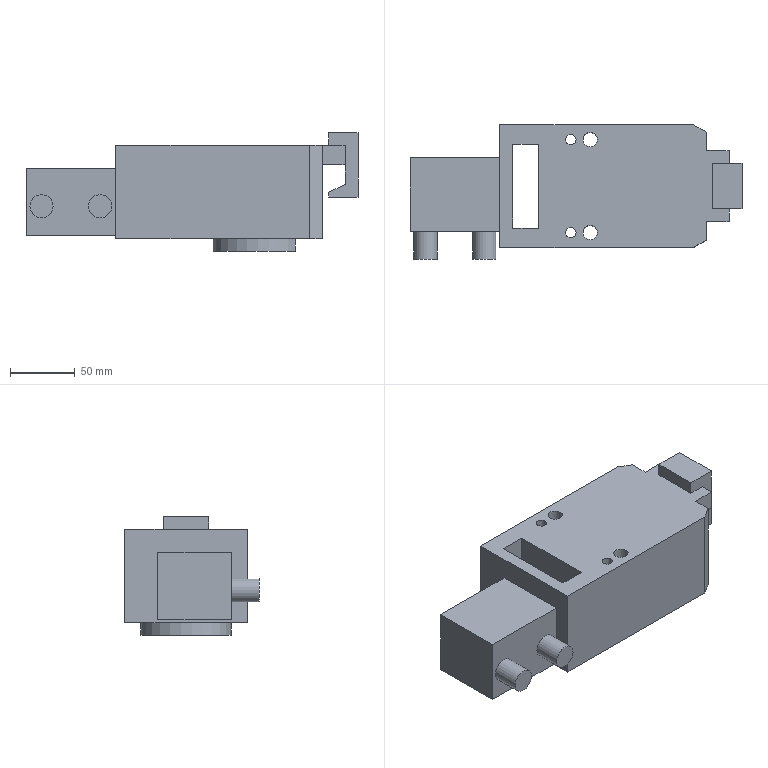Part | NX | features solid 2 | 1 solid | 46 faces | box 257 x 104 x 92 mm | volume 1265438 mm3 | plane 37 | cylinder 9 | commonest cylinder face diameters 8 x2 11 x2 17 x2 18 x2 70 x1
STEP:
#1=CARTESIAN_POINT('',(509.903,-203.405,153.));
#2=VERTEX_POINT('',#1);
#3=CARTESIAN_POINT('',(509.903,-164.213,153.));
#4=VERTEX_POINT('',#3);
#5=CARTESIAN_POINT('',(509.903,-183.809,153.));
#6=DIRECTION('',(0.,1.,0.));
#7=VECTOR('',#6,1000.);
#8=LINE('',#5,#7);
#9=EDGE_CURVE('',#2,#4,#8,.T.);
#10=ORIENTED_EDGE('',*,*,#9,.T.);
#11=CARTESIAN_POINT('',(480.903,-183.809,153.));
#12=DIRECTION('',(0.,0.,1.));
#13=DIRECTION('',(-1.,0.,0.));
#14=AXIS2_PLACEMENT_3D('',#11,#12,#13);
#15=CIRCLE('',#14,35.);
#16=EDGE_CURVE('',#4,#2,#15,.T.);
#17=ORIENTED_EDGE('',*,*,#16,.T.);
#18=EDGE_LOOP('',(#10,#17));
#19=FACE_BOUND('',#18,.T.);
#20=CARTESIAN_POINT('',(400.903,-216.309,153.));
#21=VERTEX_POINT('',#20);
#22=CARTESIAN_POINT('',(380.903,-216.309,153.));
#23=VERTEX_POINT('',#22);
#24=CARTESIAN_POINT('',(400.903,-216.309,153.));
#25=DIRECTION('',(-1.,0.,0.));
#26=VECTOR('',#25,1000.);
#27=LINE('',#24,#26);
#28=EDGE_CURVE('',#21,#23,#27,.T.);
#29=ORIENTED_EDGE('',*,*,#28,.F.);
#30=CARTESIAN_POINT('',(400.903,-151.309,153.));
#31=VERTEX_POINT('',#30);
#32=CARTESIAN_POINT('',(400.903,-156.809,153.));
#33=DIRECTION('',(0.,-1.,0.));
#34=VECTOR('',#33,1000.);
#35=LINE('',#32,#34);
#36=EDGE_CURVE('',#31,#21,#35,.T.);
#37=ORIENTED_EDGE('',*,*,#36,.F.);
#38=CARTESIAN_POINT('',(380.903,-151.309,153.));
#39=VERTEX_POINT('',#38);
#40=CARTESIAN_POINT('',(400.903,-151.309,153.));
#41=DIRECTION('',(-1.,0.,0.));
#42=VECTOR('',#41,1000.);
#43=LINE('',#40,#42);
#44=EDGE_CURVE('',#31,#39,#43,.T.);
#45=ORIENTED_EDGE('',*,*,#44,.T.);
#46=CARTESIAN_POINT('',(380.903,-156.809,153.));
#47=DIRECTION('',(0.,1.,0.));
#48=VECTOR('',#47,1000.);
#49=LINE('',#46,#48);
#50=EDGE_CURVE('',#23,#39,#49,.T.);
#51=ORIENTED_EDGE('',*,*,#50,.F.);
#52=EDGE_LOOP('',(#29,#37,#45,#51));
#53=FACE_BOUND('',#52,.T.);
#54=CARTESIAN_POINT('',(520.903,-231.309,153.));
#55=VERTEX_POINT('',#54);
#56=CARTESIAN_POINT('',(370.903,-231.309,153.));
#57=VERTEX_POINT('',#56);
#58=CARTESIAN_POINT('',(450.903,-231.309,153.));
#59=DIRECTION('',(-1.,0.,0.));
#60=VECTOR('',#59,1000.);
#61=LINE('',#58,#60);
#62=EDGE_CURVE('',#55,#57,#61,.T.);
#63=ORIENTED_EDGE('',*,*,#62,.T.);
#64=CARTESIAN_POINT('',(370.903,-136.309,153.));
#65=VERTEX_POINT('',#64);
#66=CARTESIAN_POINT('',(370.903,-156.809,153.));
#67=DIRECTION('',(0.,-1.,0.));
#68=VECTOR('',#67,1000.);
#69=LINE('',#66,#68);
#70=EDGE_CURVE('',#65,#57,#69,.T.);
#71=ORIENTED_EDGE('',*,*,#70,.F.);
#72=CARTESIAN_POINT('',(520.903,-136.309,153.));
#73=VERTEX_POINT('',#72);
#74=CARTESIAN_POINT('',(450.903,-136.309,153.));
#75=DIRECTION('',(-1.,0.,0.));
#76=VECTOR('',#75,1000.);
#77=LINE('',#74,#76);
#78=EDGE_CURVE('',#73,#65,#77,.T.);
#79=ORIENTED_EDGE('',*,*,#78,.F.);
#80=CARTESIAN_POINT('',(530.903,-142.082,153.));
#81=VERTEX_POINT('',#80);
#82=CARTESIAN_POINT('',(550.903,-153.629,153.));
#83=DIRECTION('',(0.866,-0.5,0.));
#84=VECTOR('',#83,1000.);
#85=LINE('',#82,#84);
#86=EDGE_CURVE('',#81,#73,#85,.F.);
#87=ORIENTED_EDGE('',*,*,#86,.F.);
#88=CARTESIAN_POINT('',(530.903,-225.535,153.));
#89=VERTEX_POINT('',#88);
#90=CARTESIAN_POINT('',(530.903,-178.809,153.));
#91=DIRECTION('',(0.,1.,0.));
#92=VECTOR('',#91,1000.);
#93=LINE('',#90,#92);
#94=EDGE_CURVE('',#89,#81,#93,.T.);
#95=ORIENTED_EDGE('',*,*,#94,.F.);
#96=CARTESIAN_POINT('',(520.903,-231.309,153.));
#97=DIRECTION('',(0.866,0.5,0.));
#98=VECTOR('',#97,1000.);
#99=LINE('',#96,#98);
#100=EDGE_CURVE('',#55,#89,#99,.T.);
#101=ORIENTED_EDGE('',*,*,#100,.F.);
#102=EDGE_LOOP('',(#63,#71,#79,#87,#95,#101));
#103=FACE_BOUND('',#102,.T.);
#104=CARTESIAN_POINT('',(429.903,-219.809,153.));
#105=VERTEX_POINT('',#104);
#106=CARTESIAN_POINT('',(425.903,-219.809,153.));
#107=DIRECTION('',(0.,0.,-1.));
#108=DIRECTION('',(1.,0.,0.));
#109=AXIS2_PLACEMENT_3D('',#106,#107,#108);
#110=CIRCLE('',#109,4.);
#111=EDGE_CURVE('',#105,#105,#110,.F.);
#112=ORIENTED_EDGE('',*,*,#111,.T.);
#113=EDGE_LOOP('',(#112));
#114=FACE_BOUND('',#113,.T.);
#115=CARTESIAN_POINT('',(449.403,-219.809,153.));
#116=VERTEX_POINT('',#115);
#117=CARTESIAN_POINT('',(440.903,-219.809,153.));
#118=DIRECTION('',(0.,0.,-1.));
#119=DIRECTION('',(1.,0.,0.));
#120=AXIS2_PLACEMENT_3D('',#117,#118,#119);
#121=CIRCLE('',#120,8.5);
#122=EDGE_CURVE('',#116,#116,#121,.T.);
#123=ORIENTED_EDGE('',*,*,#122,.F.);
#124=EDGE_LOOP('',(#123));
#125=FACE_BOUND('',#124,.T.);
#126=CARTESIAN_POINT('',(449.403,-147.809,153.));
#127=VERTEX_POINT('',#126);
#128=CARTESIAN_POINT('',(440.903,-147.809,153.));
#129=DIRECTION('',(0.,0.,-1.));
#130=DIRECTION('',(1.,0.,0.));
#131=AXIS2_PLACEMENT_3D('',#128,#129,#130);
#132=CIRCLE('',#131,8.5);
#133=EDGE_CURVE('',#127,#127,#132,.T.);
#134=ORIENTED_EDGE('',*,*,#133,.F.);
#135=EDGE_LOOP('',(#134));
#136=FACE_BOUND('',#135,.T.);
#137=CARTESIAN_POINT('',(429.903,-147.809,153.));
#138=VERTEX_POINT('',#137);
#139=CARTESIAN_POINT('',(425.903,-147.809,153.));
#140=DIRECTION('',(0.,0.,-1.));
#141=DIRECTION('',(1.,0.,0.));
#142=AXIS2_PLACEMENT_3D('',#139,#140,#141);
#143=CIRCLE('',#142,4.);
#144=EDGE_CURVE('',#138,#138,#143,.F.);
#145=ORIENTED_EDGE('',*,*,#144,.T.);
#146=EDGE_LOOP('',(#145));
#147=FACE_BOUND('',#146,.T.);
#148=CARTESIAN_POINT('',(400.903,-156.809,153.));
#149=DIRECTION('',(0.,0.,-1.));
#150=DIRECTION('',(1.,0.,0.));
#151=AXIS2_PLACEMENT_3D('',#148,#149,#150);
#152=PLANE('',#151);
#153=ADVANCED_FACE('',(#19,#53,#103,#114,#125,#136,#147),#152,.T.);
#154=CARTESIAN_POINT('',(400.903,-151.309,225.));
#155=VERTEX_POINT('',#154);
#156=CARTESIAN_POINT('',(400.903,-216.309,225.));
#157=VERTEX_POINT('',#156);
#158=CARTESIAN_POINT('',(400.903,-156.809,225.));
#159=DIRECTION('',(0.,-1.,0.));
#160=VECTOR('',#159,1000.);
#161=LINE('',#158,#160);
#162=EDGE_CURVE('',#155,#157,#161,.T.);
#163=ORIENTED_EDGE('',*,*,#162,.T.);
#164=CARTESIAN_POINT('',(380.903,-216.309,225.));
#165=VERTEX_POINT('',#164);
#166=CARTESIAN_POINT('',(385.903,-216.309,225.));
#167=DIRECTION('',(1.,0.,0.));
#168=VECTOR('',#167,1000.);
#169=LINE('',#166,#168);
#170=EDGE_CURVE('',#157,#165,#169,.F.);
#171=ORIENTED_EDGE('',*,*,#170,.T.);
#172=CARTESIAN_POINT('',(380.903,-151.309,225.));
#173=VERTEX_POINT('',#172);
#174=CARTESIAN_POINT('',(380.903,-156.809,225.));
#175=DIRECTION('',(0.,1.,0.));
#176=VECTOR('',#175,1000.);
#177=LINE('',#174,#176);
#178=EDGE_CURVE('',#165,#173,#177,.T.);
#179=ORIENTED_EDGE('',*,*,#178,.T.);
#180=CARTESIAN_POINT('',(385.903,-151.309,225.));
#181=DIRECTION('',(1.,0.,0.));
#182=VECTOR('',#181,1000.);
#183=LINE('',#180,#182);
#184=EDGE_CURVE('',#155,#173,#183,.F.);
#185=ORIENTED_EDGE('',*,*,#184,.F.);
#186=EDGE_LOOP('',(#163,#171,#179,#185));
#187=FACE_BOUND('',#186,.T.);
#188=CARTESIAN_POINT('',(535.903,-201.309,225.));
#189=VERTEX_POINT('',#188);
#190=CARTESIAN_POINT('',(535.903,-166.309,225.));
#191=VERTEX_POINT('',#190);
#192=CARTESIAN_POINT('',(535.903,-156.809,225.));
#193=DIRECTION('',(0.,-1.,0.));
#194=VECTOR('',#193,1000.);
#195=LINE('',#192,#194);
#196=EDGE_CURVE('',#189,#191,#195,.F.);
#197=ORIENTED_EDGE('',*,*,#196,.T.);
#198=CARTESIAN_POINT('',(548.403,-166.309,225.));
#199=VERTEX_POINT('',#198);
#200=CARTESIAN_POINT('',(568.403,-166.309,225.));
#201=DIRECTION('',(1.,0.,0.));
#202=VECTOR('',#201,1000.);
#203=LINE('',#200,#202);
#204=EDGE_CURVE('',#199,#191,#203,.F.);
#205=ORIENTED_EDGE('',*,*,#204,.F.);
#206=CARTESIAN_POINT('',(548.403,-156.309,225.));
#207=VERTEX_POINT('',#206);
#208=CARTESIAN_POINT('',(548.403,-156.809,225.));
#209=DIRECTION('',(0.,1.,0.));
#210=VECTOR('',#209,1000.);
#211=LINE('',#208,#210);
#212=EDGE_CURVE('',#199,#207,#211,.T.);
#213=ORIENTED_EDGE('',*,*,#212,.T.);
#214=CARTESIAN_POINT('',(530.903,-156.309,225.));
#215=VERTEX_POINT('',#214);
#216=CARTESIAN_POINT('',(578.403,-156.309,225.));
#217=DIRECTION('',(1.,0.,0.));
#218=VECTOR('',#217,1000.);
#219=LINE('',#216,#218);
#220=EDGE_CURVE('',#215,#207,#219,.T.);
#221=ORIENTED_EDGE('',*,*,#220,.F.);
#222=CARTESIAN_POINT('',(530.903,-142.082,225.));
#223=VERTEX_POINT('',#222);
#224=CARTESIAN_POINT('',(530.903,-178.809,225.));
#225=DIRECTION('',(0.,1.,0.));
#226=VECTOR('',#225,1000.);
#227=LINE('',#224,#226);
#228=EDGE_CURVE('',#215,#223,#227,.T.);
#229=ORIENTED_EDGE('',*,*,#228,.T.);
#230=CARTESIAN_POINT('',(520.903,-136.309,225.));
#231=VERTEX_POINT('',#230);
#232=CARTESIAN_POINT('',(550.903,-153.629,225.));
#233=DIRECTION('',(-0.866,0.5,0.));
#234=VECTOR('',#233,1000.);
#235=LINE('',#232,#234);
#236=EDGE_CURVE('',#231,#223,#235,.F.);
#237=ORIENTED_EDGE('',*,*,#236,.F.);
#238=CARTESIAN_POINT('',(370.903,-136.309,225.));
#239=VERTEX_POINT('',#238);
#240=CARTESIAN_POINT('',(400.903,-136.309,225.));
#241=DIRECTION('',(-1.,0.,0.));
#242=VECTOR('',#241,1000.);
#243=LINE('',#240,#242);
#244=EDGE_CURVE('',#231,#239,#243,.T.);
#245=ORIENTED_EDGE('',*,*,#244,.T.);
#246=CARTESIAN_POINT('',(370.903,-231.309,225.));
#247=VERTEX_POINT('',#246);
#248=CARTESIAN_POINT('',(370.903,-156.809,225.));
#249=DIRECTION('',(0.,-1.,0.));
#250=VECTOR('',#249,1000.);
#251=LINE('',#248,#250);
#252=EDGE_CURVE('',#239,#247,#251,.T.);
#253=ORIENTED_EDGE('',*,*,#252,.T.);
#254=CARTESIAN_POINT('',(520.903,-231.309,225.));
#255=VERTEX_POINT('',#254);
#256=CARTESIAN_POINT('',(400.903,-231.309,225.));
#257=DIRECTION('',(-1.,0.,0.));
#258=VECTOR('',#257,1000.);
#259=LINE('',#256,#258);
#260=EDGE_CURVE('',#255,#247,#259,.T.);
#261=ORIENTED_EDGE('',*,*,#260,.F.);
#262=CARTESIAN_POINT('',(530.903,-225.535,225.));
#263=VERTEX_POINT('',#262);
#264=CARTESIAN_POINT('',(520.903,-231.309,225.));
#265=DIRECTION('',(-0.866,-0.5,0.));
#266=VECTOR('',#265,1000.);
#267=LINE('',#264,#266);
#268=EDGE_CURVE('',#263,#255,#267,.T.);
#269=ORIENTED_EDGE('',*,*,#268,.F.);
#270=CARTESIAN_POINT('',(530.903,-211.309,225.));
#271=VERTEX_POINT('',#270);
#272=CARTESIAN_POINT('',(530.903,-178.809,225.));
#273=DIRECTION('',(0.,1.,0.));
#274=VECTOR('',#273,1000.);
#275=LINE('',#272,#274);
#276=EDGE_CURVE('',#263,#271,#275,.T.);
#277=ORIENTED_EDGE('',*,*,#276,.T.);
#278=CARTESIAN_POINT('',(548.403,-211.309,225.));
#279=VERTEX_POINT('',#278);
#280=CARTESIAN_POINT('',(578.403,-211.309,225.));
#281=DIRECTION('',(1.,0.,0.));
#282=VECTOR('',#281,1000.);
#283=LINE('',#280,#282);
#284=EDGE_CURVE('',#271,#279,#283,.T.);
#285=ORIENTED_EDGE('',*,*,#284,.T.);
#286=CARTESIAN_POINT('',(548.403,-201.309,225.));
#287=VERTEX_POINT('',#286);
#288=CARTESIAN_POINT('',(548.403,-156.809,225.));
#289=DIRECTION('',(0.,1.,0.));
#290=VECTOR('',#289,1000.);
#291=LINE('',#288,#290);
#292=EDGE_CURVE('',#279,#287,#291,.T.);
#293=ORIENTED_EDGE('',*,*,#292,.T.);
#294=CARTESIAN_POINT('',(568.403,-201.309,225.));
#295=DIRECTION('',(1.,0.,0.));
#296=VECTOR('',#295,1000.);
#297=LINE('',#294,#296);
#298=EDGE_CURVE('',#287,#189,#297,.F.);
#299=ORIENTED_EDGE('',*,*,#298,.T.);
#300=EDGE_LOOP('',(#197,#205,#213,#221,#229,#237,#245,#253,#261,#269,#277,#285,#293,#299));
#301=FACE_BOUND('',#300,.T.);
#302=CARTESIAN_POINT('',(446.403,-219.809,225.));
#303=VERTEX_POINT('',#302);
#304=CARTESIAN_POINT('',(440.903,-219.809,225.));
#305=DIRECTION('',(0.,0.,-1.));
#306=DIRECTION('',(1.,0.,0.));
#307=AXIS2_PLACEMENT_3D('',#304,#305,#306);
#308=CIRCLE('',#307,5.5);
#309=EDGE_CURVE('',#303,#303,#308,.F.);
#310=ORIENTED_EDGE('',*,*,#309,.F.);
#311=EDGE_LOOP('',(#310));
#312=FACE_BOUND('',#311,.T.);
#313=CARTESIAN_POINT('',(429.903,-219.809,225.));
#314=VERTEX_POINT('',#313);
#315=CARTESIAN_POINT('',(425.903,-219.809,225.));
#316=DIRECTION('',(0.,0.,1.));
#317=DIRECTION('',(1.,0.,0.));
#318=AXIS2_PLACEMENT_3D('',#315,#316,#317);
#319=CIRCLE('',#318,4.);
#320=EDGE_CURVE('',#314,#314,#319,.T.);
#321=ORIENTED_EDGE('',*,*,#320,.F.);
#322=EDGE_LOOP('',(#321));
#323=FACE_BOUND('',#322,.T.);
#324=CARTESIAN_POINT('',(429.903,-147.809,225.));
#325=VERTEX_POINT('',#324);
#326=CARTESIAN_POINT('',(425.903,-147.809,225.));
#327=DIRECTION('',(0.,0.,1.));
#328=DIRECTION('',(1.,0.,0.));
#329=AXIS2_PLACEMENT_3D('',#326,#327,#328);
#330=CIRCLE('',#329,4.);
#331=EDGE_CURVE('',#325,#325,#330,.T.);
#332=ORIENTED_EDGE('',*,*,#331,.F.);
#333=EDGE_LOOP('',(#332));
#334=FACE_BOUND('',#333,.T.);
#335=CARTESIAN_POINT('',(446.403,-147.809,225.));
#336=VERTEX_POINT('',#335);
#337=CARTESIAN_POINT('',(440.903,-147.809,225.));
#338=DIRECTION('',(0.,0.,-1.));
#339=DIRECTION('',(1.,0.,0.));
#340=AXIS2_PLACEMENT_3D('',#337,#338,#339);
#341=CIRCLE('',#340,5.5);
#342=EDGE_CURVE('',#336,#336,#341,.F.);
#343=ORIENTED_EDGE('',*,*,#342,.F.);
#344=EDGE_LOOP('',(#343));
#345=FACE_BOUND('',#344,.T.);
#346=CARTESIAN_POINT('',(400.903,-156.809,225.));
#347=DIRECTION('',(0.,0.,-1.));
#348=DIRECTION('',(1.,0.,0.));
#349=AXIS2_PLACEMENT_3D('',#346,#347,#348);
#350=PLANE('',#349);
#351=ADVANCED_FACE('',(#187,#301,#312,#323,#334,#345),#350,.F.);
#352=ORIENTED_EDGE('',*,*,#94,.T.);
#353=CARTESIAN_POINT('',(530.903,-142.082,225.));
#354=DIRECTION('',(0.,0.,1.));
#355=VECTOR('',#354,1000.);
#356=LINE('',#353,#355);
#357=EDGE_CURVE('',#223,#81,#356,.F.);
#358=ORIENTED_EDGE('',*,*,#357,.F.);
#359=ORIENTED_EDGE('',*,*,#228,.F.);
#360=CARTESIAN_POINT('',(530.903,-156.309,210.));
#361=VERTEX_POINT('',#360);
#362=CARTESIAN_POINT('',(530.903,-156.309,225.));
#363=DIRECTION('',(0.,0.,1.));
#364=VECTOR('',#363,1000.);
#365=LINE('',#362,#364);
#366=EDGE_CURVE('',#215,#361,#365,.F.);
#367=ORIENTED_EDGE('',*,*,#366,.T.);
#368=CARTESIAN_POINT('',(530.903,-211.309,210.));
#369=VERTEX_POINT('',#368);
#370=CARTESIAN_POINT('',(530.903,-231.309,210.));
#371=DIRECTION('',(0.,-1.,0.));
#372=VECTOR('',#371,1000.);
#373=LINE('',#370,#372);
#374=EDGE_CURVE('',#361,#369,#373,.T.);
#375=ORIENTED_EDGE('',*,*,#374,.T.);
#376=CARTESIAN_POINT('',(530.903,-211.309,225.));
#377=DIRECTION('',(0.,0.,1.));
#378=VECTOR('',#377,1000.);
#379=LINE('',#376,#378);
#380=EDGE_CURVE('',#369,#271,#379,.T.);
#381=ORIENTED_EDGE('',*,*,#380,.T.);
#382=ORIENTED_EDGE('',*,*,#276,.F.);
#383=CARTESIAN_POINT('',(530.903,-225.535,225.));
#384=DIRECTION('',(0.,0.,1.));
#385=VECTOR('',#384,1000.);
#386=LINE('',#383,#385);
#387=EDGE_CURVE('',#89,#263,#386,.T.);
#388=ORIENTED_EDGE('',*,*,#387,.F.);
#389=EDGE_LOOP('',(#352,#358,#359,#367,#375,#381,#382,#388));
#390=FACE_BOUND('',#389,.T.);
#391=CARTESIAN_POINT('',(530.903,-178.809,225.));
#392=DIRECTION('',(1.,0.,0.));
#393=DIRECTION('',(0.,1.,0.));
#394=AXIS2_PLACEMENT_3D('',#391,#392,#393);
#395=PLANE('',#394);
#396=ADVANCED_FACE('',(#390),#395,.T.);
#397=CARTESIAN_POINT('',(400.903,-216.309,225.));
#398=DIRECTION('',(0.,0.,-1.));
#399=VECTOR('',#398,1000.);
#400=LINE('',#397,#399);
#401=EDGE_CURVE('',#157,#21,#400,.T.);
#402=ORIENTED_EDGE('',*,*,#401,.F.);
#403=ORIENTED_EDGE('',*,*,#162,.F.);
#404=CARTESIAN_POINT('',(400.903,-151.309,225.));
#405=DIRECTION('',(0.,0.,-1.));
#406=VECTOR('',#405,1000.);
#407=LINE('',#404,#406);
#408=EDGE_CURVE('',#155,#31,#407,.T.);
#409=ORIENTED_EDGE('',*,*,#408,.T.);
#410=ORIENTED_EDGE('',*,*,#36,.T.);
#411=EDGE_LOOP('',(#402,#403,#409,#410));
#412=FACE_BOUND('',#411,.T.);
#413=CARTESIAN_POINT('',(400.903,-156.809,225.));
#414=DIRECTION('',(-1.,0.,0.));
#415=DIRECTION('',(0.,-1.,0.));
#416=AXIS2_PLACEMENT_3D('',#413,#414,#415);
#417=PLANE('',#416);
#418=ADVANCED_FACE('',(#412),#417,.T.);
#419=CARTESIAN_POINT('',(370.903,-218.809,207.5));
#420=VERTEX_POINT('',#419);
#421=CARTESIAN_POINT('',(370.903,-161.809,207.5));
#422=VERTEX_POINT('',#421);
#423=CARTESIAN_POINT('',(370.903,-241.309,207.5));
#424=DIRECTION('',(0.,1.,0.));
#425=VECTOR('',#424,1000.);
#426=LINE('',#423,#425);
#427=EDGE_CURVE('',#420,#422,#426,.T.);
#428=ORIENTED_EDGE('',*,*,#427,.F.);
#429=CARTESIAN_POINT('',(370.903,-218.809,155.5));
#430=VERTEX_POINT('',#429);
#431=CARTESIAN_POINT('',(370.903,-218.809,196.));
#432=DIRECTION('',(0.,0.,-1.));
#433=VECTOR('',#432,1000.);
#434=LINE('',#431,#433);
#435=EDGE_CURVE('',#420,#430,#434,.T.);
#436=ORIENTED_EDGE('',*,*,#435,.T.);
#437=CARTESIAN_POINT('',(370.903,-161.809,155.5));
#438=VERTEX_POINT('',#437);
#439=CARTESIAN_POINT('',(370.903,-146.809,155.5));
#440=DIRECTION('',(0.,-1.,0.));
#441=VECTOR('',#440,1000.);
#442=LINE('',#439,#441);
#443=EDGE_CURVE('',#438,#430,#442,.T.);
#444=ORIENTED_EDGE('',*,*,#443,.F.);
#445=CARTESIAN_POINT('',(370.903,-161.809,196.));
#446=DIRECTION('',(0.,0.,-1.));
#447=VECTOR('',#446,1000.);
#448=LINE('',#445,#447);
#449=EDGE_CURVE('',#422,#438,#448,.T.);
#450=ORIENTED_EDGE('',*,*,#449,.F.);
#451=EDGE_LOOP('',(#428,#436,#444,#450));
#452=FACE_BOUND('',#451,.T.);
#453=CARTESIAN_POINT('',(370.903,-231.309,225.));
#454=DIRECTION('',(0.,0.,-1.));
#455=VECTOR('',#454,1000.);
#456=LINE('',#453,#455);
#457=EDGE_CURVE('',#247,#57,#456,.T.);
#458=ORIENTED_EDGE('',*,*,#457,.F.);
#459=ORIENTED_EDGE('',*,*,#252,.F.);
#460=CARTESIAN_POINT('',(370.903,-136.309,225.));
#461=DIRECTION('',(0.,0.,-1.));
#462=VECTOR('',#461,1000.);
#463=LINE('',#460,#462);
#464=EDGE_CURVE('',#239,#65,#463,.T.);
#465=ORIENTED_EDGE('',*,*,#464,.T.);
#466=ORIENTED_EDGE('',*,*,#70,.T.);
#467=EDGE_LOOP('',(#458,#459,#465,#466));
#468=FACE_BOUND('',#467,.T.);
#469=CARTESIAN_POINT('',(370.903,-121.309,193.));
#470=DIRECTION('',(1.,0.,0.));
#471=DIRECTION('',(0.,0.,-1.));
#472=AXIS2_PLACEMENT_3D('',#469,#470,#471);
#473=PLANE('',#472);
#474=ADVANCED_FACE('',(#452,#468),#473,.F.);
#475=ORIENTED_EDGE('',*,*,#50,.T.);
#476=CARTESIAN_POINT('',(380.903,-151.309,193.));
#477=DIRECTION('',(0.,0.,1.));
#478=VECTOR('',#477,1000.);
#479=LINE('',#476,#478);
#480=EDGE_CURVE('',#39,#173,#479,.T.);
#481=ORIENTED_EDGE('',*,*,#480,.T.);
#482=ORIENTED_EDGE('',*,*,#178,.F.);
#483=CARTESIAN_POINT('',(380.903,-216.309,193.));
#484=DIRECTION('',(0.,0.,-1.));
#485=VECTOR('',#484,1000.);
#486=LINE('',#483,#485);
#487=EDGE_CURVE('',#165,#23,#486,.T.);
#488=ORIENTED_EDGE('',*,*,#487,.T.);
#489=EDGE_LOOP('',(#475,#481,#482,#488));
#490=FACE_BOUND('',#489,.T.);
#491=CARTESIAN_POINT('',(380.903,-235.809,193.));
#492=DIRECTION('',(-1.,0.,0.));
#493=DIRECTION('',(0.,0.,1.));
#494=AXIS2_PLACEMENT_3D('',#491,#492,#493);
#495=PLANE('',#494);
#496=ADVANCED_FACE('',(#490),#495,.F.);
#497=CARTESIAN_POINT('',(558.403,-201.309,185.));
#498=VERTEX_POINT('',#497);
#499=CARTESIAN_POINT('',(558.403,-166.309,185.));
#500=VERTEX_POINT('',#499);
#501=CARTESIAN_POINT('',(558.403,-231.309,185.));
#502=DIRECTION('',(0.,1.,0.));
#503=VECTOR('',#502,1000.);
#504=LINE('',#501,#503);
#505=EDGE_CURVE('',#498,#500,#504,.T.);
#506=ORIENTED_EDGE('',*,*,#505,.T.);
#507=CARTESIAN_POINT('',(558.403,-166.309,235.));
#508=VERTEX_POINT('',#507);
#509=CARTESIAN_POINT('',(558.403,-166.309,225.));
#510=DIRECTION('',(0.,0.,-1.));
#511=VECTOR('',#510,1000.);
#512=LINE('',#509,#511);
#513=EDGE_CURVE('',#508,#500,#512,.T.);
#514=ORIENTED_EDGE('',*,*,#513,.F.);
#515=CARTESIAN_POINT('',(558.403,-201.309,235.));
#516=VERTEX_POINT('',#515);
#517=CARTESIAN_POINT('',(558.403,-231.309,235.));
#518=DIRECTION('',(0.,1.,0.));
#519=VECTOR('',#518,1000.);
#520=LINE('',#517,#519);
#521=EDGE_CURVE('',#516,#508,#520,.T.);
#522=ORIENTED_EDGE('',*,*,#521,.F.);
#523=CARTESIAN_POINT('',(558.403,-201.309,225.));
#524=DIRECTION('',(0.,0.,1.));
#525=VECTOR('',#524,1000.);
#526=LINE('',#523,#525);
#527=EDGE_CURVE('',#516,#498,#526,.F.);
#528=ORIENTED_EDGE('',*,*,#527,.T.);
#529=EDGE_LOOP('',(#506,#514,#522,#528));
#530=FACE_BOUND('',#529,.T.);
#531=CARTESIAN_POINT('',(558.403,-231.309,225.));
#532=DIRECTION('',(1.,0.,0.));
#533=DIRECTION('',(0.,1.,0.));
#534=AXIS2_PLACEMENT_3D('',#531,#532,#533);
#535=PLANE('',#534);
#536=ADVANCED_FACE('',(#530),#535,.T.);
#537=ORIENTED_EDGE('',*,*,#521,.T.);
#538=CARTESIAN_POINT('',(535.903,-166.309,235.));
#539=VERTEX_POINT('',#538);
#540=CARTESIAN_POINT('',(578.403,-166.309,235.));
#541=DIRECTION('',(-1.,0.,0.));
#542=VECTOR('',#541,1000.);
#543=LINE('',#540,#542);
#544=EDGE_CURVE('',#508,#539,#543,.T.);
#545=ORIENTED_EDGE('',*,*,#544,.T.);
#546=CARTESIAN_POINT('',(535.903,-201.309,235.));
#547=VERTEX_POINT('',#546);
#548=CARTESIAN_POINT('',(535.903,-231.309,235.));
#549=DIRECTION('',(0.,-1.,0.));
#550=VECTOR('',#549,1000.);
#551=LINE('',#548,#550);
#552=EDGE_CURVE('',#547,#539,#551,.F.);
#553=ORIENTED_EDGE('',*,*,#552,.F.);
#554=CARTESIAN_POINT('',(578.403,-201.309,235.));
#555=DIRECTION('',(1.,0.,0.));
#556=VECTOR('',#555,1000.);
#557=LINE('',#554,#556);
#558=EDGE_CURVE('',#516,#547,#557,.F.);
#559=ORIENTED_EDGE('',*,*,#558,.F.);
#560=EDGE_LOOP('',(#537,#545,#553,#559));
#561=FACE_BOUND('',#560,.T.);
#562=CARTESIAN_POINT('',(578.403,-231.309,235.));
#563=DIRECTION('',(0.,0.,-1.));
#564=DIRECTION('',(-1.,0.,0.));
#565=AXIS2_PLACEMENT_3D('',#562,#563,#564);
#566=PLANE('',#565);
#567=ADVANCED_FACE('',(#561),#566,.F.);
#568=CARTESIAN_POINT('',(548.403,-211.309,210.));
#569=VERTEX_POINT('',#568);
#570=CARTESIAN_POINT('',(548.403,-201.309,210.));
#571=VERTEX_POINT('',#570);
#572=CARTESIAN_POINT('',(548.403,-231.309,210.));
#573=DIRECTION('',(0.,1.,0.));
#574=VECTOR('',#573,1000.);
#575=LINE('',#572,#574);
#576=EDGE_CURVE('',#569,#571,#575,.T.);
#577=ORIENTED_EDGE('',*,*,#576,.F.);
#578=CARTESIAN_POINT('',(578.403,-211.309,210.));
#579=DIRECTION('',(1.,0.,0.));
#580=VECTOR('',#579,1000.);
#581=LINE('',#578,#580);
#582=EDGE_CURVE('',#369,#569,#581,.T.);
#583=ORIENTED_EDGE('',*,*,#582,.F.);
#584=ORIENTED_EDGE('',*,*,#374,.F.);
#585=CARTESIAN_POINT('',(548.403,-156.309,210.));
#586=VERTEX_POINT('',#585);
#587=CARTESIAN_POINT('',(578.403,-156.309,210.));
#588=DIRECTION('',(-1.,0.,0.));
#589=VECTOR('',#588,1000.);
#590=LINE('',#587,#589);
#591=EDGE_CURVE('',#361,#586,#590,.F.);
#592=ORIENTED_EDGE('',*,*,#591,.T.);
#593=CARTESIAN_POINT('',(548.403,-166.309,210.));
#594=VERTEX_POINT('',#593);
#595=CARTESIAN_POINT('',(548.403,-231.309,210.));
#596=DIRECTION('',(0.,1.,0.));
#597=VECTOR('',#596,1000.);
#598=LINE('',#595,#597);
#599=EDGE_CURVE('',#594,#586,#598,.T.);
#600=ORIENTED_EDGE('',*,*,#599,.F.);
#601=CARTESIAN_POINT('',(548.403,-231.309,210.));
#602=DIRECTION('',(0.,-1.,0.));
#603=VECTOR('',#602,1000.);
#604=LINE('',#601,#603);
#605=EDGE_CURVE('',#571,#594,#604,.F.);
#606=ORIENTED_EDGE('',*,*,#605,.F.);
#607=EDGE_LOOP('',(#577,#583,#584,#592,#600,#606));
#608=FACE_BOUND('',#607,.T.);
#609=CARTESIAN_POINT('',(578.403,-231.309,210.));
#610=DIRECTION('',(0.,0.,-1.));
#611=DIRECTION('',(0.,1.,0.));
#612=AXIS2_PLACEMENT_3D('',#609,#610,#611);
#613=PLANE('',#612);
#614=ADVANCED_FACE('',(#608),#613,.T.);
#615=ORIENTED_EDGE('',*,*,#605,.T.);
#616=CARTESIAN_POINT('',(548.403,-166.309,195.));
#617=VERTEX_POINT('',#616);
#618=CARTESIAN_POINT('',(548.403,-166.309,225.));
#619=DIRECTION('',(0.,0.,1.));
#620=VECTOR('',#619,1000.);
#621=LINE('',#618,#620);
#622=EDGE_CURVE('',#594,#617,#621,.F.);
#623=ORIENTED_EDGE('',*,*,#622,.T.);
#624=CARTESIAN_POINT('',(548.403,-201.309,195.));
#625=VERTEX_POINT('',#624);
#626=CARTESIAN_POINT('',(548.403,-138.809,195.));
#627=DIRECTION('',(0.,1.,0.));
#628=VECTOR('',#627,1000.);
#629=LINE('',#626,#628);
#630=EDGE_CURVE('',#617,#625,#629,.F.);
#631=ORIENTED_EDGE('',*,*,#630,.T.);
#632=CARTESIAN_POINT('',(548.403,-201.309,225.));
#633=DIRECTION('',(0.,0.,-1.));
#634=VECTOR('',#633,1000.);
#635=LINE('',#632,#634);
#636=EDGE_CURVE('',#571,#625,#635,.T.);
#637=ORIENTED_EDGE('',*,*,#636,.F.);
#638=EDGE_LOOP('',(#615,#623,#631,#637));
#639=FACE_BOUND('',#638,.T.);
#640=CARTESIAN_POINT('',(548.403,-231.309,225.));
#641=DIRECTION('',(1.,0.,0.));
#642=DIRECTION('',(0.,1.,0.));
#643=AXIS2_PLACEMENT_3D('',#640,#641,#642);
#644=PLANE('',#643);
#645=ADVANCED_FACE('',(#639),#644,.F.);
#646=CARTESIAN_POINT('',(535.903,-201.309,185.));
#647=VERTEX_POINT('',#646);
#648=CARTESIAN_POINT('',(578.403,-201.309,185.));
#649=DIRECTION('',(1.,0.,0.));
#650=VECTOR('',#649,1000.);
#651=LINE('',#648,#650);
#652=EDGE_CURVE('',#498,#647,#651,.F.);
#653=ORIENTED_EDGE('',*,*,#652,.T.);
#654=CARTESIAN_POINT('',(535.903,-166.309,185.));
#655=VERTEX_POINT('',#654);
#656=CARTESIAN_POINT('',(535.903,-231.309,185.));
#657=DIRECTION('',(0.,-1.,0.));
#658=VECTOR('',#657,1000.);
#659=LINE('',#656,#658);
#660=EDGE_CURVE('',#655,#647,#659,.T.);
#661=ORIENTED_EDGE('',*,*,#660,.F.);
#662=CARTESIAN_POINT('',(578.403,-166.309,185.));
#663=DIRECTION('',(-1.,0.,0.));
#664=VECTOR('',#663,1000.);
#665=LINE('',#662,#664);
#666=EDGE_CURVE('',#500,#655,#665,.T.);
#667=ORIENTED_EDGE('',*,*,#666,.F.);
#668=ORIENTED_EDGE('',*,*,#505,.F.);
#669=EDGE_LOOP('',(#653,#661,#667,#668));
#670=FACE_BOUND('',#669,.T.);
#671=CARTESIAN_POINT('',(578.403,-231.309,185.));
#672=DIRECTION('',(0.,0.,-1.));
#673=DIRECTION('',(-1.,0.,0.));
#674=AXIS2_PLACEMENT_3D('',#671,#672,#673);
#675=PLANE('',#674);
#676=ADVANCED_FACE('',(#670),#675,.T.);
#677=CARTESIAN_POINT('',(535.903,-201.309,188.75));
#678=VERTEX_POINT('',#677);
#679=CARTESIAN_POINT('',(568.403,-201.309,205.));
#680=DIRECTION('',(-0.8944,0.,-0.4472));
#681=VECTOR('',#680,1000.);
#682=LINE('',#679,#681);
#683=EDGE_CURVE('',#678,#625,#682,.F.);
#684=ORIENTED_EDGE('',*,*,#683,.T.);
#685=ORIENTED_EDGE('',*,*,#630,.F.);
#686=CARTESIAN_POINT('',(535.903,-166.309,188.75));
#687=VERTEX_POINT('',#686);
#688=CARTESIAN_POINT('',(568.403,-166.309,205.));
#689=DIRECTION('',(-0.8944,0.,-0.4472));
#690=VECTOR('',#689,1000.);
#691=LINE('',#688,#690);
#692=EDGE_CURVE('',#617,#687,#691,.T.);
#693=ORIENTED_EDGE('',*,*,#692,.T.);
#694=CARTESIAN_POINT('',(535.903,-138.809,188.75));
#695=DIRECTION('',(0.,1.,0.));
#696=VECTOR('',#695,1000.);
#697=LINE('',#694,#696);
#698=EDGE_CURVE('',#678,#687,#697,.T.);
#699=ORIENTED_EDGE('',*,*,#698,.F.);
#700=EDGE_LOOP('',(#684,#685,#693,#699));
#701=FACE_BOUND('',#700,.T.);
#702=CARTESIAN_POINT('',(568.403,-138.809,205.));
#703=DIRECTION('',(-0.4472,0.,0.8944));
#704=DIRECTION('',(0.8944,0.,0.4472));
#705=AXIS2_PLACEMENT_3D('',#702,#703,#704);
#706=PLANE('',#705);
#707=ADVANCED_FACE('',(#701),#706,.T.);
#708=ORIENTED_EDGE('',*,*,#698,.T.);
#709=CARTESIAN_POINT('',(535.903,-166.309,225.));
#710=DIRECTION('',(0.,0.,-1.));
#711=VECTOR('',#710,1000.);
#712=LINE('',#709,#711);
#713=EDGE_CURVE('',#687,#655,#712,.T.);
#714=ORIENTED_EDGE('',*,*,#713,.T.);
#715=ORIENTED_EDGE('',*,*,#660,.T.);
#716=CARTESIAN_POINT('',(535.903,-201.309,225.));
#717=DIRECTION('',(0.,0.,-1.));
#718=VECTOR('',#717,1000.);
#719=LINE('',#716,#718);
#720=EDGE_CURVE('',#647,#678,#719,.F.);
#721=ORIENTED_EDGE('',*,*,#720,.T.);
#722=EDGE_LOOP('',(#708,#714,#715,#721));
#723=FACE_BOUND('',#722,.T.);
#724=CARTESIAN_POINT('',(535.903,-231.309,225.));
#725=DIRECTION('',(1.,0.,0.));
#726=DIRECTION('',(0.,1.,0.));
#727=AXIS2_PLACEMENT_3D('',#724,#725,#726);
#728=PLANE('',#727);
#729=ADVANCED_FACE('',(#723),#728,.F.);
#730=ORIENTED_EDGE('',*,*,#552,.T.);
#731=CARTESIAN_POINT('',(535.903,-166.309,225.));
#732=DIRECTION('',(0.,0.,1.));
#733=VECTOR('',#732,1000.);
#734=LINE('',#731,#733);
#735=EDGE_CURVE('',#539,#191,#734,.F.);
#736=ORIENTED_EDGE('',*,*,#735,.T.);
#737=ORIENTED_EDGE('',*,*,#196,.F.);
#738=CARTESIAN_POINT('',(535.903,-201.309,225.));
#739=DIRECTION('',(0.,0.,-1.));
#740=VECTOR('',#739,1000.);
#741=LINE('',#738,#740);
#742=EDGE_CURVE('',#547,#189,#741,.T.);
#743=ORIENTED_EDGE('',*,*,#742,.F.);
#744=EDGE_LOOP('',(#730,#736,#737,#743));
#745=FACE_BOUND('',#744,.T.);
#746=CARTESIAN_POINT('',(535.903,-231.309,225.));
#747=DIRECTION('',(1.,0.,0.));
#748=DIRECTION('',(0.,1.,0.));
#749=AXIS2_PLACEMENT_3D('',#746,#747,#748);
#750=PLANE('',#749);
#751=ADVANCED_FACE('',(#745),#750,.F.);
#752=ORIENTED_EDGE('',*,*,#236,.T.);
#753=ORIENTED_EDGE('',*,*,#357,.T.);
#754=ORIENTED_EDGE('',*,*,#86,.T.);
#755=CARTESIAN_POINT('',(520.903,-136.309,225.));
#756=DIRECTION('',(0.,0.,1.));
#757=VECTOR('',#756,1000.);
#758=LINE('',#755,#757);
#759=EDGE_CURVE('',#73,#231,#758,.T.);
#760=ORIENTED_EDGE('',*,*,#759,.T.);
#761=EDGE_LOOP('',(#752,#753,#754,#760));
#762=FACE_BOUND('',#761,.T.);
#763=CARTESIAN_POINT('',(550.903,-153.629,225.));
#764=DIRECTION('',(-0.5,-0.866,0.));
#765=DIRECTION('',(0.866,-0.5,0.));
#766=AXIS2_PLACEMENT_3D('',#763,#764,#765);
#767=PLANE('',#766);
#768=ADVANCED_FACE('',(#762),#767,.F.);
#769=ORIENTED_EDGE('',*,*,#78,.T.);
#770=ORIENTED_EDGE('',*,*,#464,.F.);
#771=ORIENTED_EDGE('',*,*,#244,.F.);
#772=ORIENTED_EDGE('',*,*,#759,.F.);
#773=EDGE_LOOP('',(#769,#770,#771,#772));
#774=FACE_BOUND('',#773,.T.);
#775=CARTESIAN_POINT('',(450.903,-136.309,225.));
#776=DIRECTION('',(0.,1.,0.));
#777=DIRECTION('',(-1.,0.,0.));
#778=AXIS2_PLACEMENT_3D('',#775,#776,#777);
#779=PLANE('',#778);
#780=ADVANCED_FACE('',(#774),#779,.T.);
#781=ORIENTED_EDGE('',*,*,#144,.F.);
#782=EDGE_LOOP('',(#781));
#783=FACE_BOUND('',#782,.T.);
#784=ORIENTED_EDGE('',*,*,#331,.T.);
#785=EDGE_LOOP('',(#784));
#786=FACE_BOUND('',#785,.T.);
#787=CARTESIAN_POINT('',(425.903,-147.809,225.));
#788=DIRECTION('',(0.,0.,-1.));
#789=DIRECTION('',(1.,0.,0.));
#790=AXIS2_PLACEMENT_3D('',#787,#788,#789);
#791=CYLINDRICAL_SURFACE('',#790,4.);
#792=ADVANCED_FACE('',(#783,#786),#791,.F.);
#793=ORIENTED_EDGE('',*,*,#133,.T.);
#794=EDGE_LOOP('',(#793));
#795=FACE_BOUND('',#794,.T.);
#796=CARTESIAN_POINT('',(449.403,-147.809,166.));
#797=VERTEX_POINT('',#796);
#798=CARTESIAN_POINT('',(440.903,-147.809,166.));
#799=DIRECTION('',(0.,0.,-1.));
#800=DIRECTION('',(1.,0.,0.));
#801=AXIS2_PLACEMENT_3D('',#798,#799,#800);
#802=CIRCLE('',#801,8.5);
#803=EDGE_CURVE('',#797,#797,#802,.T.);
#804=ORIENTED_EDGE('',*,*,#803,.F.);
#805=EDGE_LOOP('',(#804));
#806=FACE_BOUND('',#805,.T.);
#807=CARTESIAN_POINT('',(440.903,-147.809,146.));
#808=DIRECTION('',(0.,0.,-1.));
#809=DIRECTION('',(1.,0.,0.));
#810=AXIS2_PLACEMENT_3D('',#807,#808,#809);
#811=CYLINDRICAL_SURFACE('',#810,8.5);
#812=ADVANCED_FACE('',(#795,#806),#811,.F.);
#813=ORIENTED_EDGE('',*,*,#342,.T.);
#814=EDGE_LOOP('',(#813));
#815=FACE_BOUND('',#814,.T.);
#816=CARTESIAN_POINT('',(446.403,-147.809,166.));
#817=VERTEX_POINT('',#816);
#818=CARTESIAN_POINT('',(440.903,-147.809,166.));
#819=DIRECTION('',(0.,0.,-1.));
#820=DIRECTION('',(1.,0.,0.));
#821=AXIS2_PLACEMENT_3D('',#818,#819,#820);
#822=CIRCLE('',#821,5.5);
#823=EDGE_CURVE('',#817,#817,#822,.F.);
#824=ORIENTED_EDGE('',*,*,#823,.F.);
#825=EDGE_LOOP('',(#824));
#826=FACE_BOUND('',#825,.T.);
#827=CARTESIAN_POINT('',(440.903,-147.809,175.));
#828=DIRECTION('',(0.,0.,-1.));
#829=DIRECTION('',(1.,0.,0.));
#830=AXIS2_PLACEMENT_3D('',#827,#828,#829);
#831=CYLINDRICAL_SURFACE('',#830,5.5);
#832=ADVANCED_FACE('',(#815,#826),#831,.F.);
#833=ORIENTED_EDGE('',*,*,#803,.T.);
#834=EDGE_LOOP('',(#833));
#835=FACE_BOUND('',#834,.T.);
#836=ORIENTED_EDGE('',*,*,#823,.T.);
#837=EDGE_LOOP('',(#836));
#838=FACE_BOUND('',#837,.T.);
#839=CARTESIAN_POINT('',(440.903,-147.809,166.));
#840=DIRECTION('',(0.,0.,-1.));
#841=DIRECTION('',(1.,0.,0.));
#842=AXIS2_PLACEMENT_3D('',#839,#840,#841);
#843=PLANE('',#842);
#844=ADVANCED_FACE('',(#835,#838),#843,.T.);
#845=ORIENTED_EDGE('',*,*,#44,.F.);
#846=ORIENTED_EDGE('',*,*,#408,.F.);
#847=ORIENTED_EDGE('',*,*,#184,.T.);
#848=ORIENTED_EDGE('',*,*,#480,.F.);
#849=EDGE_LOOP('',(#845,#846,#847,#848));
#850=FACE_BOUND('',#849,.T.);
#851=CARTESIAN_POINT('',(385.903,-151.309,193.));
#852=DIRECTION('',(0.,-1.,0.));
#853=DIRECTION('',(0.,0.,-1.));
#854=AXIS2_PLACEMENT_3D('',#851,#852,#853);
#855=PLANE('',#854);
#856=ADVANCED_FACE('',(#850),#855,.T.);
#857=CARTESIAN_POINT('',(548.403,-156.309,225.));
#858=DIRECTION('',(0.,0.,1.));
#859=VECTOR('',#858,1000.);
#860=LINE('',#857,#859);
#861=EDGE_CURVE('',#207,#586,#860,.F.);
#862=ORIENTED_EDGE('',*,*,#861,.F.);
#863=ORIENTED_EDGE('',*,*,#212,.F.);
#864=CARTESIAN_POINT('',(548.403,-166.309,225.));
#865=DIRECTION('',(0.,0.,-1.));
#866=VECTOR('',#865,1000.);
#867=LINE('',#864,#866);
#868=EDGE_CURVE('',#199,#594,#867,.T.);
#869=ORIENTED_EDGE('',*,*,#868,.T.);
#870=ORIENTED_EDGE('',*,*,#599,.T.);
#871=EDGE_LOOP('',(#862,#863,#869,#870));
#872=FACE_BOUND('',#871,.T.);
#873=CARTESIAN_POINT('',(548.403,-261.309,225.));
#874=DIRECTION('',(-1.,0.,0.));
#875=DIRECTION('',(0.,0.,1.));
#876=AXIS2_PLACEMENT_3D('',#873,#874,#875);
#877=PLANE('',#876);
#878=ADVANCED_FACE('',(#872),#877,.F.);
#879=ORIENTED_EDGE('',*,*,#220,.T.);
#880=ORIENTED_EDGE('',*,*,#861,.T.);
#881=ORIENTED_EDGE('',*,*,#591,.F.);
#882=ORIENTED_EDGE('',*,*,#366,.F.);
#883=EDGE_LOOP('',(#879,#880,#881,#882));
#884=FACE_BOUND('',#883,.T.);
#885=CARTESIAN_POINT('',(578.403,-156.309,225.));
#886=DIRECTION('',(0.,-1.,0.));
#887=DIRECTION('',(0.,0.,-1.));
#888=AXIS2_PLACEMENT_3D('',#885,#886,#887);
#889=PLANE('',#888);
#890=ADVANCED_FACE('',(#884),#889,.F.);
#891=ORIENTED_EDGE('',*,*,#713,.F.);
#892=ORIENTED_EDGE('',*,*,#692,.F.);
#893=ORIENTED_EDGE('',*,*,#622,.F.);
#894=ORIENTED_EDGE('',*,*,#868,.F.);
#895=ORIENTED_EDGE('',*,*,#204,.T.);
#896=ORIENTED_EDGE('',*,*,#735,.F.);
#897=ORIENTED_EDGE('',*,*,#544,.F.);
#898=ORIENTED_EDGE('',*,*,#513,.T.);
#899=ORIENTED_EDGE('',*,*,#666,.T.);
#900=EDGE_LOOP('',(#891,#892,#893,#894,#895,#896,#897,#898,#899));
#901=FACE_BOUND('',#900,.T.);
#902=CARTESIAN_POINT('',(578.403,-166.309,225.));
#903=DIRECTION('',(0.,1.,0.));
#904=DIRECTION('',(-1.,0.,0.));
#905=AXIS2_PLACEMENT_3D('',#902,#903,#904);
#906=PLANE('',#905);
#907=ADVANCED_FACE('',(#901),#906,.T.);
#908=ORIENTED_EDGE('',*,*,#720,.F.);
#909=ORIENTED_EDGE('',*,*,#652,.F.);
#910=ORIENTED_EDGE('',*,*,#527,.F.);
#911=ORIENTED_EDGE('',*,*,#558,.T.);
#912=ORIENTED_EDGE('',*,*,#742,.T.);
#913=ORIENTED_EDGE('',*,*,#298,.F.);
#914=CARTESIAN_POINT('',(548.403,-201.309,225.));
#915=DIRECTION('',(0.,0.,1.));
#916=VECTOR('',#915,1000.);
#917=LINE('',#914,#916);
#918=EDGE_CURVE('',#287,#571,#917,.F.);
#919=ORIENTED_EDGE('',*,*,#918,.T.);
#920=ORIENTED_EDGE('',*,*,#636,.T.);
#921=ORIENTED_EDGE('',*,*,#683,.F.);
#922=EDGE_LOOP('',(#908,#909,#910,#911,#912,#913,#919,#920,#921));
#923=FACE_BOUND('',#922,.T.);
#924=CARTESIAN_POINT('',(578.403,-201.309,225.));
#925=DIRECTION('',(0.,1.,0.));
#926=DIRECTION('',(-1.,0.,0.));
#927=AXIS2_PLACEMENT_3D('',#924,#925,#926);
#928=PLANE('',#927);
#929=ADVANCED_FACE('',(#923),#928,.F.);
#930=ORIENTED_EDGE('',*,*,#292,.F.);
#931=CARTESIAN_POINT('',(548.403,-211.309,225.));
#932=DIRECTION('',(0.,0.,-1.));
#933=VECTOR('',#932,1000.);
#934=LINE('',#931,#933);
#935=EDGE_CURVE('',#279,#569,#934,.T.);
#936=ORIENTED_EDGE('',*,*,#935,.T.);
#937=ORIENTED_EDGE('',*,*,#576,.T.);
#938=ORIENTED_EDGE('',*,*,#918,.F.);
#939=EDGE_LOOP('',(#930,#936,#937,#938));
#940=FACE_BOUND('',#939,.T.);
#941=CARTESIAN_POINT('',(548.403,-211.309,225.));
#942=DIRECTION('',(-1.,0.,0.));
#943=DIRECTION('',(0.,0.,1.));
#944=AXIS2_PLACEMENT_3D('',#941,#942,#943);
#945=PLANE('',#944);
#946=ADVANCED_FACE('',(#940),#945,.F.);
#947=ORIENTED_EDGE('',*,*,#935,.F.);
#948=ORIENTED_EDGE('',*,*,#284,.F.);
#949=ORIENTED_EDGE('',*,*,#380,.F.);
#950=ORIENTED_EDGE('',*,*,#582,.T.);
#951=EDGE_LOOP('',(#947,#948,#949,#950));
#952=FACE_BOUND('',#951,.T.);
#953=CARTESIAN_POINT('',(578.403,-211.309,225.));
#954=DIRECTION('',(0.,-1.,0.));
#955=DIRECTION('',(0.,0.,-1.));
#956=AXIS2_PLACEMENT_3D('',#953,#954,#955);
#957=PLANE('',#956);
#958=ADVANCED_FACE('',(#952),#957,.T.);
#959=ORIENTED_EDGE('',*,*,#170,.F.);
#960=ORIENTED_EDGE('',*,*,#401,.T.);
#961=ORIENTED_EDGE('',*,*,#28,.T.);
#962=ORIENTED_EDGE('',*,*,#487,.F.);
#963=EDGE_LOOP('',(#959,#960,#961,#962));
#964=FACE_BOUND('',#963,.T.);
#965=CARTESIAN_POINT('',(385.903,-216.309,193.));
#966=DIRECTION('',(0.,-1.,0.));
#967=DIRECTION('',(0.,0.,-1.));
#968=AXIS2_PLACEMENT_3D('',#965,#966,#967);
#969=PLANE('',#968);
#970=ADVANCED_FACE('',(#964),#969,.F.);
#971=ORIENTED_EDGE('',*,*,#260,.T.);
#972=ORIENTED_EDGE('',*,*,#457,.T.);
#973=ORIENTED_EDGE('',*,*,#62,.F.);
#974=CARTESIAN_POINT('',(520.903,-231.309,135.));
#975=DIRECTION('',(0.,0.,-1.));
#976=VECTOR('',#975,1000.);
#977=LINE('',#974,#976);
#978=EDGE_CURVE('',#255,#55,#977,.T.);
#979=ORIENTED_EDGE('',*,*,#978,.F.);
#980=EDGE_LOOP('',(#971,#972,#973,#979));
#981=FACE_BOUND('',#980,.T.);
#982=CARTESIAN_POINT('',(450.903,-231.309,225.));
#983=DIRECTION('',(0.,1.,0.));
#984=DIRECTION('',(-1.,0.,0.));
#985=AXIS2_PLACEMENT_3D('',#982,#983,#984);
#986=PLANE('',#985);
#987=ADVANCED_FACE('',(#981),#986,.F.);
#988=ORIENTED_EDGE('',*,*,#268,.T.);
#989=ORIENTED_EDGE('',*,*,#978,.T.);
#990=ORIENTED_EDGE('',*,*,#100,.T.);
#991=ORIENTED_EDGE('',*,*,#387,.T.);
#992=EDGE_LOOP('',(#988,#989,#990,#991));
#993=FACE_BOUND('',#992,.T.);
#994=CARTESIAN_POINT('',(520.903,-231.309,225.));
#995=DIRECTION('',(0.5,-0.866,0.));
#996=DIRECTION('',(0.866,0.5,0.));
#997=AXIS2_PLACEMENT_3D('',#994,#995,#996);
#998=PLANE('',#997);
#999=ADVANCED_FACE('',(#993),#998,.T.);
#1000=ORIENTED_EDGE('',*,*,#309,.T.);
#1001=EDGE_LOOP('',(#1000));
#1002=FACE_BOUND('',#1001,.T.);
#1003=CARTESIAN_POINT('',(446.403,-219.809,166.));
#1004=VERTEX_POINT('',#1003);
#1005=CARTESIAN_POINT('',(440.903,-219.809,166.));
#1006=DIRECTION('',(0.,0.,-1.));
#1007=DIRECTION('',(1.,0.,0.));
#1008=AXIS2_PLACEMENT_3D('',#1005,#1006,#1007);
#1009=CIRCLE('',#1008,5.5);
#1010=EDGE_CURVE('',#1004,#1004,#1009,.F.);
#1011=ORIENTED_EDGE('',*,*,#1010,.F.);
#1012=EDGE_LOOP('',(#1011));
#1013=FACE_BOUND('',#1012,.T.);
#1014=CARTESIAN_POINT('',(440.903,-219.809,175.));
#1015=DIRECTION('',(0.,0.,-1.));
#1016=DIRECTION('',(1.,0.,0.));
#1017=AXIS2_PLACEMENT_3D('',#1014,#1015,#1016);
#1018=CYLINDRICAL_SURFACE('',#1017,5.5);
#1019=ADVANCED_FACE('',(#1002,#1013),#1018,.F.);
#1020=ORIENTED_EDGE('',*,*,#111,.F.);
#1021=EDGE_LOOP('',(#1020));
#1022=FACE_BOUND('',#1021,.T.);
#1023=ORIENTED_EDGE('',*,*,#320,.T.);
#1024=EDGE_LOOP('',(#1023));
#1025=FACE_BOUND('',#1024,.T.);
#1026=CARTESIAN_POINT('',(425.903,-219.809,225.));
#1027=DIRECTION('',(0.,0.,-1.));
#1028=DIRECTION('',(1.,0.,0.));
#1029=AXIS2_PLACEMENT_3D('',#1026,#1027,#1028);
#1030=CYLINDRICAL_SURFACE('',#1029,4.);
#1031=ADVANCED_FACE('',(#1022,#1025),#1030,.F.);
#1032=ORIENTED_EDGE('',*,*,#122,.T.);
#1033=EDGE_LOOP('',(#1032));
#1034=FACE_BOUND('',#1033,.T.);
#1035=CARTESIAN_POINT('',(449.403,-219.809,166.));
#1036=VERTEX_POINT('',#1035);
#1037=CARTESIAN_POINT('',(440.903,-219.809,166.));
#1038=DIRECTION('',(0.,0.,-1.));
#1039=DIRECTION('',(1.,0.,0.));
#1040=AXIS2_PLACEMENT_3D('',#1037,#1038,#1039);
#1041=CIRCLE('',#1040,8.5);
#1042=EDGE_CURVE('',#1036,#1036,#1041,.T.);
#1043=ORIENTED_EDGE('',*,*,#1042,.F.);
#1044=EDGE_LOOP('',(#1043));
#1045=FACE_BOUND('',#1044,.T.);
#1046=CARTESIAN_POINT('',(440.903,-219.809,146.));
#1047=DIRECTION('',(0.,0.,-1.));
#1048=DIRECTION('',(1.,0.,0.));
#1049=AXIS2_PLACEMENT_3D('',#1046,#1047,#1048);
#1050=CYLINDRICAL_SURFACE('',#1049,8.5);
#1051=ADVANCED_FACE('',(#1034,#1045),#1050,.F.);
#1052=ORIENTED_EDGE('',*,*,#1042,.T.);
#1053=EDGE_LOOP('',(#1052));
#1054=FACE_BOUND('',#1053,.T.);
#1055=ORIENTED_EDGE('',*,*,#1010,.T.);
#1056=EDGE_LOOP('',(#1055));
#1057=FACE_BOUND('',#1056,.T.);
#1058=CARTESIAN_POINT('',(440.903,-219.809,166.));
#1059=DIRECTION('',(0.,0.,-1.));
#1060=DIRECTION('',(1.,0.,0.));
#1061=AXIS2_PLACEMENT_3D('',#1058,#1059,#1060);
#1062=PLANE('',#1061);
#1063=ADVANCED_FACE('',(#1054,#1057),#1062,.T.);
#1064=CARTESIAN_POINT('',(509.903,-203.405,143.));
#1065=VERTEX_POINT('',#1064);
#1066=CARTESIAN_POINT('',(509.903,-203.405,143.));
#1067=DIRECTION('',(0.,0.,1.));
#1068=VECTOR('',#1067,1000.);
#1069=LINE('',#1066,#1068);
#1070=EDGE_CURVE('',#1065,#2,#1069,.T.);
#1071=ORIENTED_EDGE('',*,*,#1070,.F.);
#1072=CARTESIAN_POINT('',(509.903,-164.213,143.));
#1073=VERTEX_POINT('',#1072);
#1074=CARTESIAN_POINT('',(509.903,-183.809,143.));
#1075=DIRECTION('',(0.,1.,0.));
#1076=VECTOR('',#1075,1000.);
#1077=LINE('',#1074,#1076);
#1078=EDGE_CURVE('',#1065,#1073,#1077,.T.);
#1079=ORIENTED_EDGE('',*,*,#1078,.T.);
#1080=CARTESIAN_POINT('',(509.903,-164.213,143.));
#1081=DIRECTION('',(0.,0.,1.));
#1082=VECTOR('',#1081,1000.);
#1083=LINE('',#1080,#1082);
#1084=EDGE_CURVE('',#4,#1073,#1083,.F.);
#1085=ORIENTED_EDGE('',*,*,#1084,.F.);
#1086=ORIENTED_EDGE('',*,*,#9,.F.);
#1087=EDGE_LOOP('',(#1071,#1079,#1085,#1086));
#1088=FACE_BOUND('',#1087,.T.);
#1089=CARTESIAN_POINT('',(509.903,-183.809,143.));
#1090=DIRECTION('',(1.,0.,0.));
#1091=DIRECTION('',(0.,1.,0.));
#1092=AXIS2_PLACEMENT_3D('',#1089,#1090,#1091);
#1093=PLANE('',#1092);
#1094=ADVANCED_FACE('',(#1088),#1093,.T.);
#1095=ORIENTED_EDGE('',*,*,#16,.F.);
#1096=ORIENTED_EDGE('',*,*,#1084,.T.);
#1097=CARTESIAN_POINT('',(480.903,-183.809,143.));
#1098=DIRECTION('',(0.,0.,1.));
#1099=DIRECTION('',(-1.,0.,0.));
#1100=AXIS2_PLACEMENT_3D('',#1097,#1098,#1099);
#1101=CIRCLE('',#1100,35.);
#1102=EDGE_CURVE('',#1073,#1065,#1101,.T.);
#1103=ORIENTED_EDGE('',*,*,#1102,.T.);
#1104=ORIENTED_EDGE('',*,*,#1070,.T.);
#1105=EDGE_LOOP('',(#1095,#1096,#1103,#1104));
#1106=FACE_BOUND('',#1105,.T.);
#1107=CARTESIAN_POINT('',(480.903,-183.809,143.));
#1108=DIRECTION('',(0.,0.,1.));
#1109=DIRECTION('',(-1.,0.,0.));
#1110=AXIS2_PLACEMENT_3D('',#1107,#1108,#1109);
#1111=CYLINDRICAL_SURFACE('',#1110,35.);
#1112=ADVANCED_FACE('',(#1106),#1111,.T.);
#1113=ORIENTED_EDGE('',*,*,#1078,.F.);
#1114=ORIENTED_EDGE('',*,*,#1102,.F.);
#1115=EDGE_LOOP('',(#1113,#1114));
#1116=FACE_BOUND('',#1115,.T.);
#1117=CARTESIAN_POINT('',(480.903,-183.809,143.));
#1118=DIRECTION('',(0.,0.,1.));
#1119=DIRECTION('',(-1.,0.,0.));
#1120=AXIS2_PLACEMENT_3D('',#1117,#1118,#1119);
#1121=PLANE('',#1120);
#1122=ADVANCED_FACE('',(#1116),#1121,.F.);
#1123=CARTESIAN_POINT('',(322.403,-218.809,178.));
#1124=VERTEX_POINT('',#1123);
#1125=CARTESIAN_POINT('',(313.403,-218.809,178.));
#1126=DIRECTION('',(0.,-1.,0.));
#1127=DIRECTION('',(1.,0.,0.));
#1128=AXIS2_PLACEMENT_3D('',#1125,#1126,#1127);
#1129=CIRCLE('',#1128,9.);
#1130=EDGE_CURVE('',#1124,#1124,#1129,.F.);
#1131=ORIENTED_EDGE('',*,*,#1130,.T.);
#1132=EDGE_LOOP('',(#1131));
#1133=FACE_BOUND('',#1132,.T.);
#1134=CARTESIAN_POINT('',(367.903,-218.809,178.));
#1135=VERTEX_POINT('',#1134);
#1136=CARTESIAN_POINT('',(358.903,-218.809,178.));
#1137=DIRECTION('',(0.,-1.,0.));
#1138=DIRECTION('',(1.,0.,0.));
#1139=AXIS2_PLACEMENT_3D('',#1136,#1137,#1138);
#1140=CIRCLE('',#1139,9.);
#1141=EDGE_CURVE('',#1135,#1135,#1140,.F.);
#1142=ORIENTED_EDGE('',*,*,#1141,.T.);
#1143=EDGE_LOOP('',(#1142));
#1144=FACE_BOUND('',#1143,.T.);
#1145=CARTESIAN_POINT('',(301.403,-218.809,207.5));
#1146=VERTEX_POINT('',#1145);
#1147=CARTESIAN_POINT('',(326.403,-218.809,207.5));
#1148=DIRECTION('',(-1.,0.,0.));
#1149=VECTOR('',#1148,1000.);
#1150=LINE('',#1147,#1149);
#1151=EDGE_CURVE('',#420,#1146,#1150,.T.);
#1152=ORIENTED_EDGE('',*,*,#1151,.T.);
#1153=CARTESIAN_POINT('',(301.403,-218.809,155.5));
#1154=VERTEX_POINT('',#1153);
#1155=CARTESIAN_POINT('',(301.403,-218.809,207.));
#1156=DIRECTION('',(0.,0.,1.));
#1157=VECTOR('',#1156,1000.);
#1158=LINE('',#1155,#1157);
#1159=EDGE_CURVE('',#1146,#1154,#1158,.F.);
#1160=ORIENTED_EDGE('',*,*,#1159,.T.);
#1161=CARTESIAN_POINT('',(326.403,-218.809,155.5));
#1162=DIRECTION('',(1.,0.,0.));
#1163=VECTOR('',#1162,1000.);
#1164=LINE('',#1161,#1163);
#1165=EDGE_CURVE('',#1154,#430,#1164,.T.);
#1166=ORIENTED_EDGE('',*,*,#1165,.T.);
#1167=ORIENTED_EDGE('',*,*,#435,.F.);
#1168=EDGE_LOOP('',(#1152,#1160,#1166,#1167));
#1169=FACE_BOUND('',#1168,.T.);
#1170=CARTESIAN_POINT('',(326.403,-218.809,207.));
#1171=DIRECTION('',(0.,-1.,0.));
#1172=DIRECTION('',(0.,0.,-1.));
#1173=AXIS2_PLACEMENT_3D('',#1170,#1171,#1172);
#1174=PLANE('',#1173);
#1175=ADVANCED_FACE('',(#1133,#1144,#1169),#1174,.T.);
#1176=CARTESIAN_POINT('',(367.903,-240.309,178.));
#1177=VERTEX_POINT('',#1176);
#1178=CARTESIAN_POINT('',(358.903,-240.309,178.));
#1179=DIRECTION('',(0.,-1.,0.));
#1180=DIRECTION('',(1.,0.,0.));
#1181=AXIS2_PLACEMENT_3D('',#1178,#1179,#1180);
#1182=CIRCLE('',#1181,9.);
#1183=EDGE_CURVE('',#1177,#1177,#1182,.F.);
#1184=ORIENTED_EDGE('',*,*,#1183,.F.);
#1185=EDGE_LOOP('',(#1184));
#1186=FACE_BOUND('',#1185,.T.);
#1187=CARTESIAN_POINT('',(358.903,-240.309,178.));
#1188=DIRECTION('',(0.,-1.,0.));
#1189=DIRECTION('',(0.,0.,1.));
#1190=AXIS2_PLACEMENT_3D('',#1187,#1188,#1189);
#1191=PLANE('',#1190);
#1192=ADVANCED_FACE('',(#1186),#1191,.T.);
#1193=ORIENTED_EDGE('',*,*,#1141,.F.);
#1194=EDGE_LOOP('',(#1193));
#1195=FACE_BOUND('',#1194,.T.);
#1196=ORIENTED_EDGE('',*,*,#1183,.T.);
#1197=EDGE_LOOP('',(#1196));
#1198=FACE_BOUND('',#1197,.T.);
#1199=CARTESIAN_POINT('',(358.903,-238.309,178.));
#1200=DIRECTION('',(0.,1.,0.));
#1201=DIRECTION('',(0.,0.,-1.));
#1202=AXIS2_PLACEMENT_3D('',#1199,#1200,#1201);
#1203=CYLINDRICAL_SURFACE('',#1202,9.);
#1204=ADVANCED_FACE('',(#1195,#1198),#1203,.T.);
#1205=CARTESIAN_POINT('',(301.403,-161.809,155.5));
#1206=VERTEX_POINT('',#1205);
#1207=CARTESIAN_POINT('',(301.403,-205.809,155.5));
#1208=DIRECTION('',(0.,-1.,0.));
#1209=VECTOR('',#1208,1000.);
#1210=LINE('',#1207,#1209);
#1211=EDGE_CURVE('',#1154,#1206,#1210,.F.);
#1212=ORIENTED_EDGE('',*,*,#1211,.T.);
#1213=CARTESIAN_POINT('',(405.903,-161.809,155.5));
#1214=DIRECTION('',(-1.,0.,0.));
#1215=VECTOR('',#1214,1000.);
#1216=LINE('',#1213,#1215);
#1217=EDGE_CURVE('',#438,#1206,#1216,.T.);
#1218=ORIENTED_EDGE('',*,*,#1217,.F.);
#1219=ORIENTED_EDGE('',*,*,#443,.T.);
#1220=ORIENTED_EDGE('',*,*,#1165,.F.);
#1221=EDGE_LOOP('',(#1212,#1218,#1219,#1220));
#1222=FACE_BOUND('',#1221,.T.);
#1223=CARTESIAN_POINT('',(405.903,-146.809,155.5));
#1224=DIRECTION('',(0.,0.,-1.));
#1225=DIRECTION('',(1.,0.,0.));
#1226=AXIS2_PLACEMENT_3D('',#1223,#1224,#1225);
#1227=PLANE('',#1226);
#1228=ADVANCED_FACE('',(#1222),#1227,.T.);
#1229=CARTESIAN_POINT('',(301.403,-161.809,207.5));
#1230=VERTEX_POINT('',#1229);
#1231=CARTESIAN_POINT('',(326.403,-161.809,207.5));
#1232=DIRECTION('',(1.,0.,0.));
#1233=VECTOR('',#1232,1000.);
#1234=LINE('',#1231,#1233);
#1235=EDGE_CURVE('',#1230,#422,#1234,.T.);
#1236=ORIENTED_EDGE('',*,*,#1235,.T.);
#1237=ORIENTED_EDGE('',*,*,#449,.T.);
#1238=ORIENTED_EDGE('',*,*,#1217,.T.);
#1239=CARTESIAN_POINT('',(301.403,-161.809,207.));
#1240=DIRECTION('',(0.,0.,1.));
#1241=VECTOR('',#1240,1000.);
#1242=LINE('',#1239,#1241);
#1243=EDGE_CURVE('',#1230,#1206,#1242,.F.);
#1244=ORIENTED_EDGE('',*,*,#1243,.F.);
#1245=EDGE_LOOP('',(#1236,#1237,#1238,#1244));
#1246=FACE_BOUND('',#1245,.T.);
#1247=CARTESIAN_POINT('',(326.403,-161.809,207.));
#1248=DIRECTION('',(0.,-1.,0.));
#1249=DIRECTION('',(0.,0.,-1.));
#1250=AXIS2_PLACEMENT_3D('',#1247,#1248,#1249);
#1251=PLANE('',#1250);
#1252=ADVANCED_FACE('',(#1246),#1251,.F.);
#1253=CARTESIAN_POINT('',(301.403,-205.809,207.5));
#1254=DIRECTION('',(0.,-1.,0.));
#1255=VECTOR('',#1254,1000.);
#1256=LINE('',#1253,#1255);
#1257=EDGE_CURVE('',#1146,#1230,#1256,.F.);
#1258=ORIENTED_EDGE('',*,*,#1257,.F.);
#1259=ORIENTED_EDGE('',*,*,#1151,.F.);
#1260=ORIENTED_EDGE('',*,*,#427,.T.);
#1261=ORIENTED_EDGE('',*,*,#1235,.F.);
#1262=EDGE_LOOP('',(#1258,#1259,#1260,#1261));
#1263=FACE_BOUND('',#1262,.T.);
#1264=CARTESIAN_POINT('',(326.403,-205.809,207.5));
#1265=DIRECTION('',(0.,0.,-1.));
#1266=DIRECTION('',(1.,0.,0.));
#1267=AXIS2_PLACEMENT_3D('',#1264,#1265,#1266);
#1268=PLANE('',#1267);
#1269=ADVANCED_FACE('',(#1263),#1268,.F.);
#1270=CARTESIAN_POINT('',(322.403,-240.309,178.));
#1271=VERTEX_POINT('',#1270);
#1272=CARTESIAN_POINT('',(313.403,-240.309,178.));
#1273=DIRECTION('',(0.,-1.,0.));
#1274=DIRECTION('',(1.,0.,0.));
#1275=AXIS2_PLACEMENT_3D('',#1272,#1273,#1274);
#1276=CIRCLE('',#1275,9.);
#1277=EDGE_CURVE('',#1271,#1271,#1276,.F.);
#1278=ORIENTED_EDGE('',*,*,#1277,.F.);
#1279=EDGE_LOOP('',(#1278));
#1280=FACE_BOUND('',#1279,.T.);
#1281=CARTESIAN_POINT('',(364.903,-240.309,178.));
#1282=DIRECTION('',(0.,-1.,0.));
#1283=DIRECTION('',(0.,0.,1.));
#1284=AXIS2_PLACEMENT_3D('',#1281,#1282,#1283);
#1285=PLANE('',#1284);
#1286=ADVANCED_FACE('',(#1280),#1285,.T.);
#1287=ORIENTED_EDGE('',*,*,#1130,.F.);
#1288=EDGE_LOOP('',(#1287));
#1289=FACE_BOUND('',#1288,.T.);
#1290=ORIENTED_EDGE('',*,*,#1277,.T.);
#1291=EDGE_LOOP('',(#1290));
#1292=FACE_BOUND('',#1291,.T.);
#1293=CARTESIAN_POINT('',(313.403,-238.309,178.));
#1294=DIRECTION('',(0.,1.,0.));
#1295=DIRECTION('',(0.,0.,-1.));
#1296=AXIS2_PLACEMENT_3D('',#1293,#1294,#1295);
#1297=CYLINDRICAL_SURFACE('',#1296,9.);
#1298=ADVANCED_FACE('',(#1289,#1292),#1297,.T.);
#1299=ORIENTED_EDGE('',*,*,#1211,.F.);
#1300=ORIENTED_EDGE('',*,*,#1159,.F.);
#1301=ORIENTED_EDGE('',*,*,#1257,.T.);
#1302=ORIENTED_EDGE('',*,*,#1243,.T.);
#1303=EDGE_LOOP('',(#1299,#1300,#1301,#1302));
#1304=FACE_BOUND('',#1303,.T.);
#1305=CARTESIAN_POINT('',(301.403,-205.809,207.));
#1306=DIRECTION('',(-1.,0.,0.));
#1307=DIRECTION('',(0.,0.,-1.));
#1308=AXIS2_PLACEMENT_3D('',#1305,#1306,#1307);
#1309=PLANE('',#1308);
#1310=ADVANCED_FACE('',(#1304),#1309,.T.);
#1311=CLOSED_SHELL('',(#153,#351,#396,#418,#474,#496,#536,#567,#614,#645,#676,#707,#729,#751,#768,#780,#792,#812,#832,#844,#856,#878,#890,#907,#929,#946,#958,#970,#987,#999,#1019,#1031,#1051,#1063,#1094,#1112,#1122,#1175,#1192,#1204,#1228,#1252,#1269,#1286,#1298,#1310));
#1312=MANIFOLD_SOLID_BREP('',#1311);
#1313=(LENGTH_UNIT()NAMED_UNIT(*)SI_UNIT(.MILLI.,.METRE.));
#1314=UNCERTAINTY_MEASURE_WITH_UNIT(LENGTH_MEASURE(0.00001),#1313,'','');
#1315=(NAMED_UNIT(*)PLANE_ANGLE_UNIT()SI_UNIT($,.RADIAN.));
#1316=(NAMED_UNIT(*)SI_UNIT($,.STERADIAN.)SOLID_ANGLE_UNIT());
#1317=(GEOMETRIC_REPRESENTATION_CONTEXT(3)GLOBAL_UNCERTAINTY_ASSIGNED_CONTEXT((#1314))GLOBAL_UNIT_ASSIGNED_CONTEXT((#1313,#1315,#1316))REPRESENTATION_CONTEXT('',''));
#1318=ADVANCED_BREP_SHAPE_REPRESENTATION('',(#1312),#1317);